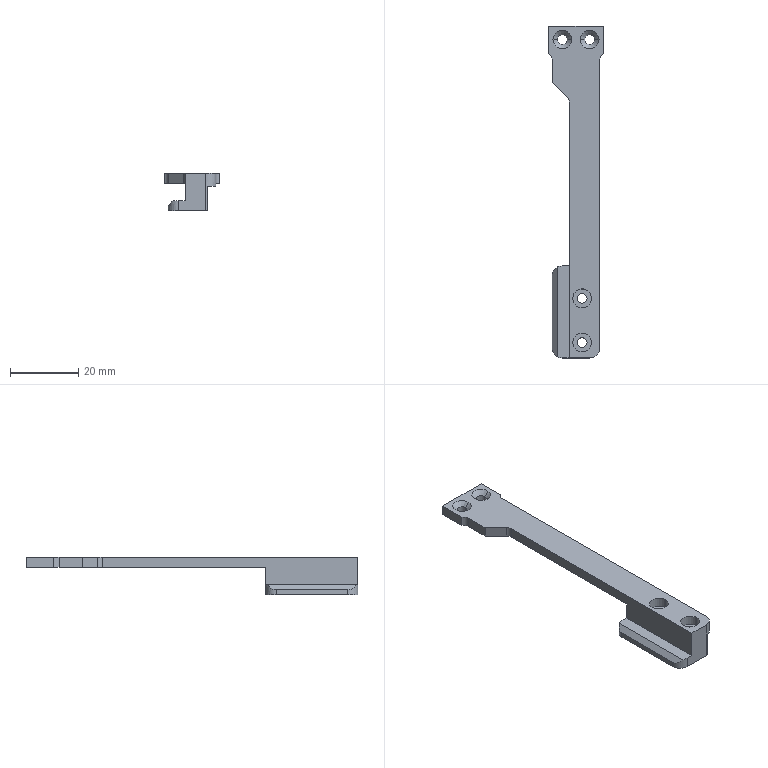NC program | NX | posted with a generic post | part box 16 x 97.4 x 11 mm
Whole program:
N10 G17 G21 G94 G90
(PLANAR_MILL , TOOL : D50面刀)
N12 T01 M6
N14 G53
N16 G17 G0 G90 X82.5 Y0. S4500 M3
N18 G43 Z20. H1
N20 Z2.
N22 G94 G1 Z0. F1000.
N24 X52.5
N26 X-52.5
N28 X-82.5
N30 Z2.
N32 G0 Z20.
N34 M5
(ADAPTIVE_MILLING , TOOL : D8-25-D8-60-3T-ROUGH)
N36 T02 M6
N38 G53
N40 G17 G0 G90 X-46.402 Y19.028 S6500 M3
N42 G43 Z20. H2
N44 Z-9.
N46 G94 G1 X-46.392 Y18.879 Z-9.937 F3000.
N48 X-46.383 Y18.729 Z-10.308
N50 X-46.373 Y18.579 Z-10.58
N52 X-46.364 Y18.429 Z-10.8
N54 X-46.354 Y18.28 Z-10.984
N56 X-46.345 Y18.13 Z-11.142
N58 X-46.335 Y17.98 Z-11.28
N60 X-46.326 Y17.831 Z-11.4
N62 X-46.316 Y17.681 Z-11.505
N64 X-46.306 Y17.531 Z-11.598
N66 X-46.297 Y17.382 Z-11.679
N68 X-46.287 Y17.232 Z-11.75
N70 X-46.278 Y17.082 Z-11.81
N72 X-46.268 Y16.932 Z-11.862
N74 X-46.259 Y16.783 Z-11.905
N76 X-46.249 Y16.633 Z-11.939
N78 X-46.24 Y16.483 Z-11.966
N80 X-46.23 Y16.334 Z-11.985
N82 X-46.221 Y16.184 Z-11.996
N84 X-46.211 Y16.034 Z-12.
N86 X-46.127 Y14.717
N88 G3 X-45.678 Y14.044 R0.808
N90 X-44.706 Y13.718 R3.559
N92 X-42.222 Y13.429 R17.156
N94 X-37.674 Y13.316 R97.009
N96 X-30.871 Y13.3 R763.382
N98 G1 X50.416 Y13.298
N100 G2 X52.463 Y12.608 R3.969
N102 X54.236 Y10.667 R5.764
N104 X55.257 Y7.88 R9.538
N106 X55.661 Y4.583 R22.23
N108 X55.783 Y0.035 R94.426
N110 X55.794 Y-8.015 R791.493
N112 X54.909 Y-10.261 R4.102
N114 X52.73 Y-11.98 R6.13
N116 X49.897 Y-12.857 R10.685
N118 X46.416 Y-13.198 R27.086
N120 X40.642 Y-13.292 R152.341
N122 G1 X34.517 Y-13.299
N124 X-50.405 Y-13.298
N126 G2 X-52.672 Y-12.474 R4.03
N128 X-54.396 Y-10.394 R5.971
N130 X-55.306 Y-7.66 R10.142
N132 X-55.685 Y-4.184 R24.685
N134 X-55.79 Y0.89 R120.171
N136 X-55.795 Y7.977 R799.405
N138 X-54.931 Y10.231 R4.082
N140 X-52.83 Y11.929 R6.022
N142 X-50.008 Y12.837 R10.358
N144 X-46.612 Y13.046 R12.952
N146 X-43.267 Y12.812 R655.851
N148 G3 X-36.446 Y12.619 R126.041
N150 X-28.071 Y12.6 R886.745
N152 G1 X48.054
N154 G2 X52.13 Y10.86 R5.749
N156 X53.837 Y8.22 R8.021
N158 X54.677 Y5.011 R13.845
N160 X55.015 Y0.827 R36.965
N162 X55.092 Y-5.734 R199.467
N164 X53.412 Y-9.583 R5.707
N166 X51.744 Y-10.847 R7.544
N168 G1 X51.634 Y-10.935
N170 X51.226 Y-11.293
N172 X50.775 Y-11.594
N174 X50.288 Y-11.834
N176 X49.774 Y-12.009
N178 G2 X47.766 Y-12.299 R17.026
N180 X42.698 Y-12.552 R62.148
N182 X32.198 Y-12.599 R684.903
N184 G1 X-48.088
N186 G2 X-52.094 Y-10.904 R5.706
N188 X-53.851 Y-8.193 R7.99
N190 X-54.696 Y-4.892 R14.186
N192 X-55.025 Y-0.531 R39.592
N194 X-55.091 Y5.768 R209.536
N196 X-53.4 Y9.598 R5.703
N198 X-50.192 Y11.518 R7.881
N200 X-47.097 Y12.055 R12.577
N202 X-43.423 Y12.069 R43.051
N204 G3 X-30.768 Y11.912 R366.289
N206 G1 X-24.818 Y11.911
N208 X-19.146 Y11.901
N210 X39.216 Y11.904
N212 X39.313 Y11.91
N214 X39.405 Y11.943
N216 G2 X40.7 Y12.15 R4.458
N218 G1 X48.7
N220 X49.242 Y12.114
N222 X49.774 Y12.008
N224 X50.288 Y11.834
N226 X50.775 Y11.594
N228 X51.227 Y11.292
N230 X51.635 Y10.934
N232 X51.993 Y10.526
N234 X52.294 Y10.075
N236 G2 X52.786 Y8.932 R7.946
N238 X54.029 Y3.576 R22.29
N240 X54.33 Y-1.313 R54.903
N242 X54.36 Y-4.113 R55.856
N244 X53.079 Y-7.871 R6.816
N246 G3 X52.823 Y-8.409 R1.194
N248 G1 X52.814 Y-8.542
N250 X52.708 Y-9.074
N252 X52.534 Y-9.588
N254 X52.294 Y-10.075
N256 X51.992 Y-10.527
N258 X51.634 Y-10.935
N260 X51.226 Y-11.293
N262 X50.775 Y-11.594
N264 X50.288 Y-11.834
N266 X49.774 Y-12.009
N268 X49.241 Y-12.115
N270 X48.7 Y-12.15
N272 X40.7
N274 G2 X39.504 Y-12.058 R26.192
N276 G3 X34.834 Y-11.917 R75.914
N278 X27.755 Y-11.912 R915.533
N280 G1 X21.195 Y-11.91
N282 X14.543 Y-11.911
N284 X8.855 Y-11.912
N286 X2.295 Y-11.91
N288 X-4.357 Y-11.911
N290 X-10.045 Y-11.912
N292 X-16.605 Y-11.91
N294 X-23.257 Y-11.911
N296 X-28.945 Y-11.912
N298 X-35.505 Y-11.91
N300 X-42.157 Y-11.911
N302 G2 X-46.445 Y-11.902 R363.082
N304 X-50.076 Y-10.787 R6.809
N306 X-52.479 Y-8.132 R7.677
N308 X-53.689 Y-4.851 R12.044
N310 X-54.21 Y-0.952 R26.009
N312 X-54.362 Y3.945 R78.972
N314 X-53.167 Y7.724 R6.66
N316 X-50.369 Y10.046 R7.311
N318 X-47.109 Y11.013 R11.338
N320 X-44.615 Y11.244 R19.109
N322 X-40.24 Y11.268 R90.415
N324 G3 X-26.496 Y11.211 R972.598
N326 G1 X-20.369 Y11.202
N328 X36.591 Y11.201
N330 G3 X37.866 Y11.22 R30.407
N332 X38.31 Y11.393 R0.897
N334 G2 X39.403 Y11.942 R4.489
N336 G3 X39.881 Y12.46 R0.8
N338 G1 X39.92 Y12.593
N340 X40.368 Y14.103 Z-11.9
N342 X40.428 Y14.308 F15000.
N344 X40.493 Y14.512
N346 G2 X41.176 Y15.012 R0.8
N348 G1 X42.32 Y15.099
N350 X43.465 Y15.18
N352 G2 X47.041 Y14.962 R15.611
N354 G1 X49.465 Y14.531
N356 G2 X52.242 Y13.617 R10.349
N358 X54.18 Y11.619 R4.161
N360 X54.698 Y10.453 R30.613
N362 X55.672 Y7.475 R20.843
N364 X56.453 Y3.624 R48.181
N366 G1 X56.843 Y1.191
N368 G2 X56.894 Y-3.677 R16.419
N370 X55.7 Y-8.423 R22.696
N372 G1 X55.145 Y-9.922
N374 G2 X53.588 Y-12.351 R6.749
N376 G1 X53.345 Y-12.594
N378 X53.1 Y-12.835
N380 G2 X51.435 Y-13.927 R5.954
N382 X49.324 Y-14.539 R8.216
N384 X47.858 Y-14.649 R9.488
N386 G1 X42.768 Y-14.633
N388 G2 X42.121 Y-14.301 R0.8
N390 G1 X41.995 Y-14.126
N392 X41.072 Y-12.849 Z-12. F3000.
N394 X40.783 Y-12.448
N396 G3 X40.261 Y-12.127 R0.8
N398 G2 X39.16 Y-11.847 R4.176
N400 G3 X37.181 Y-11.461 R10.069
N402 X33.309 Y-11.254 R43.648
N404 X24.798 Y-11.211 R537.488
N406 G1 X-43.627
N408 G2 X-45.64 Y-11.15 R20.214
N410 X-46.829 Y-11.06 R7.518
N412 G1 X-47.597 Y-10.894
N414 X-48.277 Y-10.669
N416 X-48.931 Y-10.378
N418 X-49.553 Y-10.023
N420 X-50.136 Y-9.608
N422 X-50.674 Y-9.136
N424 X-51.163 Y-8.613
N426 X-51.597 Y-8.043
N428 X-51.972 Y-7.433
N430 X-52.284 Y-6.789
N432 X-52.53 Y-6.116
N434 G2 X-53.436 Y-0.759 R28.799
N436 X-53.588 Y2.561 R37.75
N438 X-52.928 Y5.617 R7.487
N440 X-52.363 Y6.603 R7.056
N442 G3 X-52.232 Y6.908 R1.505
N444 G1 X-51.892 Y7.575
N446 X-51.484 Y8.203
N448 X-51.013 Y8.784
N450 X-50.484 Y9.314
N452 X-49.902 Y9.785
N454 X-49.275 Y10.192
N456 X-48.608 Y10.532
N458 X-47.909 Y10.8
N460 X-47.186 Y10.994
N462 X-46.668 Y11.076
N464 G3 X-46.418 Y12.573 R0.8
N466 X-46.768 Y12.669 Z-11.977 R0.911
N468 G1 X-47.968 Y12.821 Z-11.9
N470 X-49.193 Y12.976 F15000.
N472 G3 X-49.737 Y12.848 R0.801
N474 G1 X-51.376 Y11.756
N476 G3 X-52.999 Y10.279 R7.361
N478 X-53.965 Y8.863 R9.48
N480 G1 X-54.923 Y7.143
N482 G3 X-55.799 Y4.695 R7.904
N484 X-55.906 Y3.397 R7.242
N486 G1 X-55.895 Y1.82
N488 X-55.88 Y0.244
N490 X-55.858 Y-0.925
N492 X-55.826 Y-2.093
N494 X-55.776 Y-3.651
N496 G3 X-55.61 Y-4.113 R0.801
N498 G1 X-54.727 Y-5.259
N500 X-54.131 Y-6.031 Z-11.962 F3000.
N502 G3 X-53.628 Y-6.332 Z-12. R0.801
N504 X-52.707 Y-5.423 R0.8
N506 G1 X-52.814 Y-4.715
N508 X-52.85 Y-4.
N510 Y4.
N512 X-52.811 Y4.748
N514 X-52.694 Y5.487
N516 X-52.5 Y6.21
N518 X-52.232 Y6.908
N520 X-51.892 Y7.575
N522 X-51.484 Y8.203
N524 X-51.013 Y8.784
N526 X-50.484 Y9.314
N528 X-49.902 Y9.785
N530 X-49.275 Y10.192
N532 X-48.608 Y10.532
N534 X-47.909 Y10.8
N536 X-47.186 Y10.994
N538 X-46.447 Y11.111
N540 X-45.7 Y11.15
N542 X-24.7
N544 X-23.947 Y11.11
N546 X-23.203 Y10.992
N548 G3 X-21.366 Y10.7 R10.842
N550 X-17.093 Y10.529 R58.413
N552 X-9.784 Y10.501 R702.079
N554 G1 X29.679
N556 G3 X30.058 Y10.594 R0.885
N558 G1 X30.545 Y10.834
N560 X31.059 Y11.009
N562 X31.592 Y11.114
N564 X32.133 Y11.15
N566 X37.708
N568 G3 X38.296 Y11.382 R0.885
N570 X37.751 Y12.956 R0.88
N572 G1 X32.182 Y12.93
N574 X30.607 Y12.923 Z-11.9
N576 X-21.903 Y12.68 F15000.
N578 X-22.377 Y12.679 Z-11.93 F3000.
N580 X-22.851 Y12.673 Z-11.96
N582 G3 X-23.415 Y12.43 Z-12. R0.88
N584 X-23.034 Y10.946 R0.88
N586 G1 X-22.475 Y10.795
N588 G3 X-21.284 Y10.376 R10.102
N590 X-18.624 Y9.989 R15.901
N592 X-13.776 Y9.825 R80.03
N594 X-7.159 Y9.802 R706.917
N596 G1 X27.657
N598 G3 X28.961 Y9.88 R8.911
N600 X29.317 Y10.038 R1.004
N602 G1 X29.607 Y10.293
N604 X30.044 Y10.584
N606 G3 X30.324 Y11.743 R0.88
N608 X29.555 Y12.196 Z-11.941 R0.88
N610 G1 X28.915 Z-11.9
N612 X-20.696 Y12.186 F15000.
N614 X-21.054 Y12.187 Z-11.923 F3000.
N616 X-21.412 Y12.184 Z-11.945
N618 G3 X-22.122 Y11.764 Z-12. R0.88
N620 X-21.773 Y10.523 R0.88
N622 X-20.751 Y10.019 R15.197
N624 X-18.845 Y9.527 R9.403
N626 X-15.327 Y9.215 R31.139
N628 X-8.639 Y9.107 R177.423
N630 G1 X-4.796 Y9.102
N632 X26.157 Y9.103
N634 G3 X27.842 Y9.182 R15.371
N636 X28.525 Y9.335 R2.58
N638 X28.732 Y9.468 R1.803
N640 G2 X29.33 Y10.05 R9.159
N642 G3 X29.518 Y11.141 R0.88
N644 X28.754 Y11.592 Z-11.941 R0.88
N646 G1 X28.109 Y11.594 Z-11.9
N648 X-19.968 Y11.792 F15000.
N650 X-20.616 Y11.795 Z-11.941 F3000.
N652 G3 X-21.383 Y11.353 Z-12. R0.88
N654 X-21.102 Y10.179 R0.88
N656 X-20.29 Y9.659 R17.383
N658 X-18.517 Y9.038 R6.961
N660 X-15.312 Y8.609 R21.922
N662 X-10.183 Y8.432 R89.515
N664 X-2.521 Y8.402 R733.617
N666 G1 X24.673 Y8.403
N668 G3 X26.915 Y8.495 R22.789
N670 X27.862 Y8.686 R4.037
N672 X28.088 Y8.823 R1.617
N674 G1 X28.768 Y9.504
N676 G3 X28.909 Y10.565 R0.88
N678 X28.152 Y11.006 Z-11.942 R0.883
N680 G1 X27.493 Y11.011 Z-11.9
N682 X-19.264 Y11.323 F15000.
N684 X-19.909 Y11.327 Z-11.941 F3000.
N686 G3 X-20.679 Y10.884 Z-12. R0.88
N688 X-20.472 Y9.766 R0.88
N690 G1 X-19.93 Y9.323
N692 G3 X-18.391 Y8.609 R5.466
N694 X-15.594 Y8.062 R15.768
N696 X-11.092 Y7.781 R52.593
N698 X-2.78 Y7.704 R329.295
N700 G1 X1.417 Y7.702
N702 X22.762 Y7.703
N704 G3 X25.767 Y7.78 R40.305
N706 X27.147 Y8.005 R6.74
N708 X27.436 Y8.171 R1.061
N710 G1 X28.116 Y8.852
N712 G3 X28.258 Y9.91 R0.88
N714 X27.504 Y10.354 Z-11.942 R0.883
N716 G1 X26.845 Y10.362 Z-11.9
N718 X-18.716 Y10.877 F15000.
N720 X-19.363 Y10.884 Z-11.941 F3000.
N722 G3 X-20.133 Y10.447 Z-12. R0.88
N724 X-19.93 Y9.323 R0.88
N726 G1 X-19.581 Y8.978
N728 G3 X-18.305 Y8.222 R4.452
N730 X-15.83 Y7.558 R11.893
N732 X-11.884 Y7.164 R34.848
N734 X-5.389 Y7.019 R146.421
N736 X2.992 Y7.003 R929.816
N738 G1 X21.101
N740 G3 X24.752 Y7.075 R59.004
N742 X26.441 Y7.323 R8.305
N744 X26.76 Y7.495 R1.043
N746 G1 X27.44 Y8.176
N748 G3 X27.584 Y9.231 R0.88
N750 X26.833 Y9.678 Z-11.942 R0.883
N752 G1 X26.173 Y9.69 Z-11.9
N754 X-18.278 Y10.465 F15000.
N756 X-18.63 Y10.472 Z-11.922 F3000.
N758 X-18.981 Y10.475 Z-11.945
N760 G3 X-19.705 Y10.057 Z-12. R0.88
N762 X-19.581 Y8.978 R0.88
N764 G2 X-19.249 Y8.616 R2.829
N766 G3 X-18.208 Y7.854 R3.674
N768 X-16.049 Y7.098 R9.193
N770 X-12.557 Y6.588 R24.686
N772 X-6.846 Y6.349 R84.86
N774 X5.004 Y6.303 R901.745
N776 G1 X20.05
N778 G3 X23.888 Y6.378 R65.949
N780 X25.602 Y6.602 R10.161
N782 X26.082 Y6.817 R1.095
N784 G1 X26.762 Y7.498
N786 G3 X26.908 Y8.549 R0.88
N788 X26.161 Y9. Z-11.942 R0.883
N790 G1 X25.499 Y9.016 Z-11.9
N792 X-17.857 Y10.03 F15000.
N794 X-18.219 Y10.039 Z-11.923 F3000.
N796 X-18.582 Y10.045 Z-11.946
N798 G3 X-19.297 Y9.65 Z-12. R0.88
N800 X-19.249 Y8.616 R0.88
N802 X-18.765 Y8.025 R15.651
N804 X-17.547 Y7.184 R4.353
N806 X-15.14 Y6.39 R10.85
N808 X-13.824 Y6.15 R22.321
N810 G1 X24.851
N812 G3 X25.386 Y6.235 R2.074
N814 X25.661 Y6.397 R1.09
N816 G1 X26.094 Y6.83
N818 G3 X24.977 Y8.18 R0.88
N820 G1 X24.356 Y7.758
N822 G3 X24.851 Y6.15 R0.88
N824 X25.388 Y6.214 R1.326
N826 X25.644 Y6.382 R0.947
N828 X25.887 Y7.15 R0.8
N830 G1 X25.819 Y7.455
N832 X25.473 Y8.992 Z-11.9
N834 X25.443 Y9.124 F15000.
N836 X25.417 Y9.257
N838 G2 X25.644 Y9.926 R0.8
N840 G1 X27.387 Y11.669
N842 G2 X29.853 Y13.087 R5.458
N844 X32.738 Y13.66 R23.744
N846 G1 X34.093 Y13.843
N848 X35.45 Y14.022
N850 G2 X41.543 Y14.58 R89.585
N852 G1 X46.414 Y14.859
N854 G2 X49.514 Y14.541 R9.839
N856 X52.167 Y13.601 R15.696
N858 G1 X53.452 Y13.011
N860 G2 X53.759 Y11.805 R0.8
N862 G1 X53.63 Y11.633
N864 X52.686 Y10.371 Z-12. F3000.
N866 G3 X52.493 Y9.893 R0.845
N868 X52.534 Y9.588 R0.808
N870 G1 X52.709 Y9.074
N872 X52.815 Y8.541
N874 G3 X53.114 Y5.362 R42.02
N876 G2 X53.615 Y-2.142 R71.446
N878 G1 Y-4.755
N880 G2 X53.484 Y-5.17 R1.258
N882 G1 X52.899 Y-6.492
N884 G3 X52.85 Y-6.717 R2.433
N886 G1 Y-8.
N888 X52.821 Y-8.437
N890 G3 X53.767 Y-9.275 R0.8
N892 X54.282 Y-8.938 Z-11.96 R0.806
N894 G1 X54.811 Y-8.157 Z-11.9
N896 X55.369 Y-7.333 F15000.
N898 G3 X55.507 Y-6.886 R0.801
N900 G1 X55.536 Y6.449
N902 G3 X55.391 Y6.91 R0.801
N904 G1 X54.822 Y7.721
N906 X54.305 Y8.459 Z-11.957 F3000.
N908 G3 X53.743 Y8.794 Z-12. R0.8
N910 X52.85 Y8. R0.8
N912 G1 Y0.737
N914 G2 X52.887 Y-2.189 R70.707
N916 G1 X52.85 Y-2.72
N918 Y-6.745
N920 G3 X54.213 Y-7.313 R0.8
N922 X54.402 Y-7.017 Z-11.978 R0.805
N924 G1 X54.818 Y-5.868 Z-11.9
N926 X55.309 Y-4.51 F15000.
N928 G3 X55.356 Y-4.238 R0.812
N930 G1 Y-1.769
N932 G3 X55.309 Y-1.497 R0.812
N934 G1 X54.821 Y-0.148
N936 X54.402 Y1.009 Z-11.978 F3000.
N938 G3 X54.22 Y1.299 Z-12. R0.806
N940 X52.85 Y0.737 R0.8
N942 G1 Y-2.763
N944 G3 X53.212 Y-3.432 R0.8
N946 G1 X53.5 Y-3.621
N948 X54.818 Y-4.484 Z-11.9
N950 X54.94 Y-4.563 F15000.
N952 X55.059 Y-4.646
N954 G2 X55.356 Y-5.269 R0.8
N956 G1 Y-8.222
N958 G2 X54.893 Y-10.316 R5.041
N960 X53.998 Y-11.803 R7.279
N962 G1 X53.642 Y-12.261
N964 X53.282 Y-12.716
N966 G2 X51.56 Y-13.972 R4.554
N968 X50.057 Y-14.348 R5.057
N970 X46.725 Y-14.622 R120.723
N972 G1 X45.94 Y-14.67
N974 X45.154 Y-14.712
N976 X40.932 Y-14.917
N978 G2 X40.116 Y-14.309 R0.8
N980 G1 X40.063 Y-14.092
N982 X39.686 Y-12.562 Z-12. F3000.
N984 X39.657 Y-12.445
N986 X39.625 Y-12.328
N988 G3 X39.16 Y-11.847 R0.8
N990 G2 X38.568 Y-11.559 R3.884
N992 G3 X37.454 Y-11.152 R4.266
N994 G1 X-45.691 Y-11.15
N996 G3 X-46.571 Y-12.03 R0.88
N998 X-45.695 Y-12.91 R0.88
N1000 G1 X8.024 Y-13.113
N1002 X9.599 Y-13.119 Z-11.9
N1004 X37.516 Y-13.225 F15000.
N1006 X38.168 Y-13.227 Z-11.941 F3000.
N1008 G3 X38.933 Y-12.788 Z-12. R0.88
N1010 X38.643 Y-11.604 R0.88
N1012 G2 X38.134 Y-11.265 R8.397
N1014 G3 X37.708 Y-11.15 R0.868
N1016 G1 X37.358
N1018 G3 X36.608 Y-11.657 R0.808
N1020 G1 X36.226 Y-12.612
N1022 G2 X35.476 Y-13.119 R0.808
N1024 G1 X35.326 Z-11.996
N1026 X35.176 Z-11.985
N1028 X35.026 Z-11.966
N1030 X34.876 Z-11.939
N1032 X34.726 Z-11.905
N1034 X34.576 Z-11.862
N1036 X34.426 Z-11.81
N1038 X34.276 Z-11.75
N1040 X34.126 Z-11.679
N1042 X33.976 Z-11.598
N1044 X33.826 Z-11.505
N1046 X33.676 Z-11.4
N1048 X33.526 Z-11.28
N1050 X33.376 Z-11.142
N1052 X33.226 Z-10.984
N1054 X33.076 Z-10.8
N1056 X32.926 Z-10.58
N1058 X32.776 Z-10.308
N1060 X32.626 Z-9.937
N1062 X32.476 Z-9.
N1064 G0 Z20.
N1066 X-15.046 Y10.372
N1068 Z-9.
N1070 G1 X-15.196 Y10.364 Z-9.937
N1072 X-15.346 Y10.357 Z-10.308
N1074 X-15.496 Y10.349 Z-10.58
N1076 X-15.646 Y10.342 Z-10.8
N1078 X-15.796 Y10.334 Z-10.984
N1080 X-15.945 Y10.327 Z-11.142
N1082 X-16.095 Y10.319 Z-11.28
N1084 X-16.245 Y10.312 Z-11.4
N1086 X-16.395 Y10.305 Z-11.505
N1088 X-16.545 Y10.297 Z-11.598
N1090 X-16.694 Y10.29 Z-11.679
N1092 X-16.844 Y10.282 Z-11.75
N1094 X-16.994 Y10.275 Z-11.81
N1096 X-17.144 Y10.267 Z-11.862
N1098 X-17.294 Y10.26 Z-11.905
N1100 X-17.444 Y10.253 Z-11.939
N1102 X-17.593 Y10.245 Z-11.966
N1104 X-17.743 Y10.238 Z-11.985
N1106 X-17.893 Y10.23 Z-11.996
N1108 X-18.043 Y10.223 Z-12.
N1110 G3 X-18.787 Y9.612 R0.808
N1112 G1 X-18.991 Y8.796
N1114 G3 X-18.888 Y8.164 R0.808
N1116 X-18.419 Y7.511 R4.079
N1118 X-17.057 Y6.569 R4.771
N1120 X-16.125 Y6.183 R9.402
N1122 G1 X-15.952 Y6.15
N1124 X-13.764
N1126 G3 X-12.976 Y7.421 R0.88
N1128 X-13.512 Y7.873 Z-11.954 R0.885
N1130 G1 X-14.33 Y8.118 Z-11.9
N1132 X-17.035 Y8.927 F15000.
N1134 X-17.659 Y9.113 Z-11.941 F3000.
N1136 G3 X-18.517 Y8.908 Z-12. R0.88
N1138 X-18.652 Y7.796 R0.88
N1140 G2 X-18.404 Y7.373 R2.829
N1142 G3 X-17.494 Y6.466 R3.324
N1144 X-16.956 Y6.175 R1.735
N1146 G1 X-16.806 Y6.15
N1148 X-15.931
N1150 G3 X-15.064 Y7.175 R0.88
N1152 X-15.579 Y7.836 Z-11.945 R0.883
N1154 G1 X-16.222 Y8.117 Z-11.9
N1156 X-16.669 Y8.313 F15000.
N1158 X-17.264 Y8.573 Z-11.941 F3000.
N1160 G3 X-18.142 Y8.473 Z-12. R0.88
N1162 X-18.404 Y7.373 R0.88
N1164 G1 X-18.169 Y6.903
N1166 G3 X-17.593 Y6.274 R2.
N1168 X-17.204 Y6.15 R0.98
N1170 G1 X-16.766
N1172 G3 X-16.416 Y7.837 R0.88
N1174 G1 X-17.032 Y8.104
N1176 G3 X-18.169 Y6.903 R0.88
N1178 G1 X-18.039 Y6.595
N1180 G3 X-17.296 Y6.15 R0.845
N1182 G1 X-17.121
N1184 G3 X-16.321 Y7.071 R0.808
N1186 G1 X-16.469 Y8.119
N1188 X-16.49 Y8.268 Z-11.996
N1190 X-16.511 Y8.416 Z-11.985
N1192 X-16.532 Y8.565 Z-11.966
N1194 X-16.554 Y8.713 Z-11.939
N1196 X-16.575 Y8.862 Z-11.905
N1198 X-16.596 Y9.01 Z-11.862
N1200 X-16.617 Y9.159 Z-11.81
N1202 X-16.638 Y9.307 Z-11.75
N1204 X-16.659 Y9.456 Z-11.679
N1206 X-16.68 Y9.604 Z-11.598
N1208 X-16.701 Y9.753 Z-11.505
N1210 X-16.722 Y9.901 Z-11.4
N1212 X-16.743 Y10.05 Z-11.28
N1214 X-16.764 Y10.198 Z-11.142
N1216 X-16.785 Y10.347 Z-10.984
N1218 X-16.806 Y10.495 Z-10.8
N1220 X-16.827 Y10.644 Z-10.58
N1222 X-16.848 Y10.792 Z-10.308
N1224 X-16.869 Y10.941 Z-9.937
N1226 X-16.89 Y11.089 Z-9.
N1228 G0 Z20.
(ADAPTIVE_MILLING_COPY , TOOL : D8-25-D8-60-3T-ROUGH)
N1230 X-57.78 Y0.242
N1232 Z-4.85
N1234 G1 X-57.632 Y0.266 Z-5.787
N1236 X-57.484 Y0.29 Z-6.158
N1238 X-57.335 Y0.314 Z-6.43
N1240 X-57.187 Y0.338 Z-6.65
N1242 X-57.039 Y0.362 Z-6.834
N1244 X-56.891 Y0.386 Z-6.992
N1246 X-56.743 Y0.411 Z-7.13
N1248 X-56.595 Y0.435 Z-7.25
N1250 X-56.447 Y0.459 Z-7.355
N1252 X-56.299 Y0.483 Z-7.448
N1254 X-56.151 Y0.507 Z-7.529
N1256 X-56.003 Y0.531 Z-7.6
N1258 X-55.855 Y0.555 Z-7.66
N1260 X-55.707 Y0.579 Z-7.712
N1262 X-55.559 Y0.603 Z-7.755
N1264 X-55.411 Y0.627 Z-7.789
N1266 X-55.263 Y0.651 Z-7.816
N1268 X-55.115 Y0.675 Z-7.835
N1270 X-54.967 Y0.7 Z-7.846
N1272 X-54.819 Y0.724 Z-7.85
N1274 X-53.528 Y0.934
N1276 G3 X-52.849 Y1.731 R0.808
N1278 G2 X-52.619 Y3.365 R4.604
N1280 X-51.945 Y5.342 R19.07
N1282 X-49.932 Y8.166 R7.591
N1284 X-47.33 Y9.587 R7.546
N1286 X-44.245 Y10.199 R14.819
N1288 X-40.051 Y10.412 R50.021
N1290 X-31.652 Y10.45 R543.432
N1292 X-26.196 Y10.44 R435.149
N1294 X-23.362 Y9.952 R9.242
N1296 X-20.651 Y8.229 R7.471
N1298 X-19.443 Y7.016 R224.252
N1300 G3 X-18.439 Y6.235 R5.055
N1302 X-18.122 Y6.15 R1.075
N1304 G1 X-17.247
N1306 G3 X-16.475 Y6.738 R0.8
N1308 X-16.598 Y7.418 Z-7.805 R0.805
N1310 G1 X-17.101 Y8.116 Z-7.75
N1312 X-18.081 Y9.476 F15000.
N1314 X-18.121 Y9.526
N1316 X-18.164 Y9.574
N1318 X-18.395 Y9.806
N1320 X-18.63 Y10.035
N1322 G3 X-19.278 Y10.53 R4.311
N1324 G1 X-20.008 Y10.986
N1326 X-20.742 Y11.437
N1328 G3 X-22.76 Y12.314 R9.095
N1330 X-24.201 Y12.584 R7.625
N1332 G1 X-25.344 Y12.684
N1334 X-26.487 Y12.774
N1336 G3 X-29.105 Y12.907 R71.653
N1338 G1 X-35.996 Y13.131
N1340 G3 X-43.828 Y12.688 R44.113
N1342 G1 X-44.624 Y12.572
N1344 X-45.42 Y12.451
N1346 G3 X-50.148 Y10.963 R17.847
N1348 G1 X-50.588 Y10.754
N1350 X-51.026 Y10.541
N1352 G3 X-53.482 Y8.122 R5.861
N1354 G1 X-54.391 Y6.434
N1356 G3 X-54.48 Y5.95 R0.801
N1358 G1 X-54.289 Y4.498
N1360 X-54.162 Y3.539 Z-7.811 F3000.
N1362 G3 X-53.872 Y3.021 Z-7.85 R0.8
N1364 X-52.619 Y3.365 R0.8
N1366 G2 X-52.219 Y4.2 R5.047
N1368 X-50.736 Y6.094 R19.531
N1370 X-47.039 Y8.53 R9.468
N1372 X-43.47 Y9.372 R16.153
N1374 X-39.195 Y9.676 R43.365
N1376 X-31.67 Y9.748 R275.178
N1378 X-27.558 Y9.735 R190.549
N1380 X-24.879 Y9.358 R10.668
N1382 X-22.274 Y8.113 R9.666
N1384 X-20.406 Y6.785 R61.295
N1386 G3 X-19.494 Y6.221 R7.669
N1388 X-19.215 Y6.15 R1.307
N1390 G1 X-18.078
N1392 G3 X-17.315 Y6.708 R0.8
N1394 X-17.405 Y7.383 Z-7.805 R0.8
N1396 G1 X-17.877 Y8.116 Z-7.75
N1398 X-18.612 Y9.261 F15000.
N1400 G3 X-18.995 Y9.574 R0.801
N1402 G1 X-22.659 Y11.001
N1404 G3 X-26.442 Y11.957 R15.788
N1406 X-30.356 Y12.359 R92.331
N1408 X-34.284 Y12.399 R27.92
N1410 G1 X-41.655 Y11.956
N1412 G3 X-46.928 Y11.091 R26.082
N1414 X-50.857 Y9.324 R14.319
N1416 G1 X-52.831 Y8.05
N1418 G3 X-53.196 Y7.415 R0.8
N1420 G1 X-53.258 Y6.078
N1422 X-53.299 Y5.208 Z-7.805 F3000.
N1424 G3 X-53.037 Y4.578 Z-7.85 R0.8
N1426 X-51.913 Y4.626 R0.8
N1428 G2 X-51.154 Y5.347 R4.836
N1430 X-48.936 Y6.706 R36.392
N1432 X-44.164 Y8.378 R16.329
N1434 X-39.647 Y8.891 R33.34
N1436 X-33.262 Y9.038 R132.904
N1438 X-28.887 Y9.033 R185.583
N1440 X-25.944 Y8.646 R12.409
N1442 X-22.888 Y7.359 R13.485
N1444 G3 X-21.105 Y6.354 R103.956
N1446 X-20.601 Y6.156 R1.661
N1448 X-19.154 Y6.15 R44.718
N1450 X-18.355 Y7.003 R0.8
N1452 X-18.678 Y7.593 Z-7.806 R0.8
N1454 G1 X-19.387 Y8.117 Z-7.75
N1456 X-20.742 Y9.118 F15000.
N1458 G3 X-20.926 Y9.219 R0.85
N1460 G1 X-23.669 Y10.295
N1462 G3 X-27.837 Y11.364 R17.649
N1464 X-31.362 Y11.55 R22.075
N1466 G1 X-38.585 Y11.352
N1468 G3 X-43.791 Y10.863 R39.475
N1470 G1 X-44.339 Y10.775
N1472 X-44.886 Y10.683
N1474 G3 X-48.086 Y9.749 R16.188
N1476 G1 X-49.794 Y9.053
N1478 G3 X-50.118 Y8.811 R0.803
N1480 G1 X-51.04 Y7.655
N1482 X-51.68 Y6.851 Z-7.815 F3000.
N1484 G3 X-51.854 Y6.343 Z-7.85 R0.801
N1486 X-50.712 Y5.63 R0.8
N1488 G2 X-49.654 Y6.039 R4.744
N1490 G3 X-47.425 Y6.732 R58.634
N1492 G2 X-40.827 Y8.031 R30.548
N1494 X-34.972 Y8.305 R79.506
N1496 X-29.985 Y8.323 R135.921
N1498 X-24.303 Y7.054 R14.468
N1500 G1 X-22.448 Y6.214
N1502 G3 X-22.186 Y6.15 R1.555
N1504 G1 X-20.524
N1506 G3 X-19.728 Y7.033 R0.8
N1508 X-20.064 Y7.605 Z-7.807 R0.8
N1510 G1 X-20.793 Y8.117 Z-7.75
N1512 X-21.61 Y8.691 F15000.
N1514 G3 X-22.074 Y8.836 R0.801
N1516 G1 X-48.188 Y8.704
N1518 G3 X-48.618 Y8.576 R0.802
N1520 G1 X-49.385 Y8.081
N1522 X-50.323 Y7.476 Z-7.821 F3000.
N1524 G3 X-50.619 Y7.133 Z-7.85 R0.802
N1526 X-49.739 Y6.018 R0.8
N1528 G2 X-48.612 Y6.15 R4.791
N1530 G3 X-46.585 Y6.418 R16.153
N1532 G2 X-42.268 Y7.117 R76.734
N1534 X-35.811 Y7.56 R67.754
N1536 X-30.999 Y7.604 R96.322
N1538 X-25.266 Y6.507 R17.413
N1540 G1 X-24.343 Y6.175
N1542 X-24.195 Y6.15
N1544 X-22.182
N1546 G3 X-21.387 Y7.034 R0.8
N1548 X-21.723 Y7.605 Z-7.807 R0.8
N1550 G1 X-22.454 Y8.117 Z-7.75
N1552 X-23.274 Y8.691 F15000.
N1554 G3 X-23.733 Y8.836 R0.801
N1556 G1 X-47.062
N1558 G3 X-47.521 Y8.691 R0.801
N1560 G1 X-48.333 Y8.122
N1562 X-49.071 Y7.605 Z-7.807 F3000.
N1564 G3 X-49.407 Y7.044 Z-7.85 R0.8
N1566 X-48.612 Y6.15 R0.8
N1568 X-45.641 Y6.156 R263.886
N1570 X-42.506 Y6.412 R64.3
N1572 G2 X-32.196 Y6.884 R99.248
N1574 X-27.009 Y6.173 R20.625
N1576 G1 X-26.874 Y6.15
N1578 X-24.162
N1580 G3 X-23.908 Y7.709 R0.8
N1582 G1 X-25.43 Y8.118 Z-7.75
N1584 X-26.169 Y8.316 F15000.
N1586 X-26.261 Y8.334
N1588 X-26.354 Y8.343
N1590 X-44.262 Y8.836
N1592 G3 X-44.747 Y8.688 R0.801
N1594 G1 X-45.543 Y8.122
N1596 X-46.276 Y7.602 Z-7.807 F3000.
N1598 G3 X-46.608 Y7.035 Z-7.85 R0.8
N1600 X-45.812 Y6.15 R0.8
N1602 G1 X-26.825
N1604 G3 X-26.025 Y6.845 R0.808
N1606 G1 X-25.846 Y8.119
N1608 X-25.825 Y8.268 Z-7.846
N1610 X-25.804 Y8.416 Z-7.835
N1612 X-25.783 Y8.565 Z-7.816
N1614 X-25.762 Y8.713 Z-7.789
N1616 X-25.741 Y8.862 Z-7.755
N1618 X-25.72 Y9.01 Z-7.712
N1620 X-25.699 Y9.159 Z-7.66
N1622 X-25.679 Y9.307 Z-7.6
N1624 X-25.658 Y9.456 Z-7.529
N1626 X-25.637 Y9.604 Z-7.448
N1628 X-25.616 Y9.753 Z-7.355
N1630 X-25.595 Y9.902 Z-7.25
N1632 X-25.574 Y10.05 Z-7.13
N1634 X-25.553 Y10.199 Z-6.992
N1636 X-25.532 Y10.347 Z-6.834
N1638 X-25.511 Y10.496 Z-6.65
N1640 X-25.491 Y10.644 Z-6.43
N1642 X-25.47 Y10.793 Z-6.158
N1644 X-25.449 Y10.941 Z-5.787
N1646 X-25.428 Y11.09 Z-4.85
N1648 G0 Z20.
N1650 M5
(DRILLING , TOOL : 倒角D6-90度)
N1652 T03 M6
N1654 G53
N1656 G17 G0 G90 X-44.2 Y-1.799 S2500 M3
N1658 G43 Z20. H3
N1660 G94 G81 G99 Z-2.85 F200. R3.
N1662 X-31.2
N1664 G80
N1666 G0 X-31.2 Y-1.799 Z20.
(DRILLING_COPY , TOOL : 倒角D6-90度)
N1668 X44.7 Y-4.
N1670 G81 Z-2.75 F200. R3.
N1672 Y4.
N1674 G80
N1676 G0 X44.7 Y4. Z20.
(PLANAR_MILL_4 , TOOL : 倒角D6-90度)
N1678 X-52.798 Y8. S3000
N1680 Z-8.5
N1682 G1 Z-10.5 F600.
N1684 X-48.298
N1686 X-22.102
N1688 X-17.602
N1690 Z-8.5
N1692 G0 Z20.
(PLANAR_MILL_3_COPY_1 , TOOL : 倒角D6-90度)
N1694 X42.613 Y-11.992 S3500
N1696 Z0.5
N1698 G1 Z-1.5 F1000.
N1700 G41 X42.7 Y-11.5 D3
N1702 G3 X40.7 Y-9.5 R2.
N1704 G2 X39.401 Y-8.75 R1.5
N1706 G3 X38.968 Y-8.5 R0.5
N1708 G1 X-45.7
N1710 G2 X-50.2 Y-4. R4.5
N1712 G1 Y2.
N1714 G2 X-48.7 Y3.5 R1.5
N1716 G1 X26.305
N1718 G3 X26.658 Y3.646 R0.5
N1720 G1 X31.072 Y8.061
N1722 G2 X32.133 Y8.5 R1.5
N1724 G1 X38.968
N1726 G3 X39.401 Y8.75 R0.5
N1728 G2 X40.7 Y9.5 R1.5
N1730 G1 X48.7
N1732 G2 X50.2 Y8. R1.5
N1734 G1 Y-8.
N1736 G2 X48.7 Y-9.5 R1.5
N1738 G1 X40.7
N1740 G3 X38.7 Y-11.5 R2.
N1742 G40
N1744 G1 X38.787 Y-11.992
N1746 Z0.5
N1748 G0 Z20.
N1750 M5
(DRILLING_COPY_1 , TOOL : 钻头D2.9-39-67)
N1752 T04 M6
N1754 G53
N1756 G17 G0 G90 X-44.2 Y-1.799 S3000 M3
N1758 G43 Z20. H4
N1760 G94 G83 G99 Z-15. F200. Q2. R3.
N1762 X-31.2
N1764 G80
N1766 G0 X-31.2 Y-1.799 Z20.
(DRILLING_COPY_COPY , TOOL : 钻头D2.9-39-67)
N1768 X44.7 Y-4.
N1770 G81 Z-6. F200. R3.
N1772 Y4.
N1774 G80
N1776 G0 X44.7 Y4. Z20.
N1778 M5
(PLANAR_MILL_1 , TOOL : D3-9-D4-50-3T-ROUGH)
N1780 T05 M6
N1782 G53
N1784 G17 G0 G90 X-43.324 Y-0.96 S4500 M3
N1786 G43 Z20. H5
N1788 Z0.5
N1790 G94 G1 X-43.337 Y-0.936 Z0.499 F800.
N1792 X-43.931 Y-0.609 Z0.469
N1794 X-44.469 Z0.446
N1796 X-45.063 Y-0.936 Z0.416
N1798 X-45.39 Y-1.53 Z0.387
N1800 Y-2.068 Z0.363
N1802 X-45.063 Y-2.662 Z0.333
N1804 X-44.469 Y-2.989 Z0.304
N1806 X-43.931 Z0.28
N1808 X-43.337 Y-2.662 Z0.251
N1810 X-43.01 Y-2.068 Z0.221
N1812 Y-1.53 Z0.198
N1814 X-43.337 Y-0.936 Z0.168
N1816 X-43.931 Y-0.609 Z0.138
N1818 X-44.469 Z0.115
N1820 X-45.063 Y-0.936 Z0.085
N1822 X-45.39 Y-1.53 Z0.056
N1824 Y-2.068 Z0.032
N1826 X-45.063 Y-2.662 Z0.003
N1828 X-44.469 Y-2.989 Z-0.027
N1830 X-43.931 Z-0.05
N1832 X-43.337 Y-2.662 Z-0.08
N1834 X-43.01 Y-2.068 Z-0.11
N1836 Y-1.53 Z-0.133
N1838 X-43.337 Y-0.936 Z-0.163
N1840 X-43.931 Y-0.609 Z-0.192
N1842 X-44.469 Z-0.216
N1844 X-45.063 Y-0.936 Z-0.245
N1846 X-45.39 Y-1.53 Z-0.275
N1848 Y-2.068 Z-0.298
N1850 X-45.063 Y-2.662 Z-0.328
N1852 X-44.469 Y-2.989 Z-0.358
N1854 X-43.931 Z-0.381
N1856 X-43.337 Y-2.662 Z-0.411
N1858 X-43.01 Y-2.068 Z-0.44
N1860 Y-1.53 Z-0.464
N1862 X-43.337 Y-0.936 Z-0.493
N1864 X-43.931 Y-0.609 Z-0.523
N1866 X-44.469 Z-0.547
N1868 X-45.063 Y-0.936 Z-0.576
N1870 X-45.39 Y-1.53 Z-0.606
N1872 Y-2.068 Z-0.629
N1874 X-45.063 Y-2.662 Z-0.659
N1876 X-44.469 Y-2.989 Z-0.688
N1878 X-43.931 Z-0.712
N1880 X-43.337 Y-2.662 Z-0.741
N1882 X-43.01 Y-2.068 Z-0.771
N1884 Y-1.53 Z-0.795
N1886 X-43.337 Y-0.936 Z-0.824
N1888 X-43.931 Y-0.609 Z-0.854
N1890 X-44.469 Z-0.877
N1892 X-45.063 Y-0.936 Z-0.907
N1894 X-45.39 Y-1.53 Z-0.936
N1896 Y-2.068 Z-0.96
N1898 X-45.063 Y-2.662 Z-0.99
N1900 X-44.469 Y-2.989 Z-1.019
N1902 X-43.931 Z-1.043
N1904 X-43.337 Y-2.662 Z-1.072
N1906 X-43.01 Y-2.068 Z-1.102
N1908 Y-1.53 Z-1.125
N1910 X-43.337 Y-0.936 Z-1.155
N1912 X-43.931 Y-0.609 Z-1.185
N1914 X-44.469 Z-1.208
N1916 X-45.063 Y-0.936 Z-1.238
N1918 X-45.39 Y-1.53 Z-1.267
N1920 Y-2.068 Z-1.291
N1922 X-45.063 Y-2.662 Z-1.32
N1924 X-44.469 Y-2.989 Z-1.35
N1926 X-43.931 Z-1.373
N1928 X-43.337 Y-2.662 Z-1.403
N1930 X-43.01 Y-2.068 Z-1.433
N1932 Y-1.53 Z-1.456
N1934 X-43.337 Y-0.936 Z-1.486
N1936 X-43.931 Y-0.609 Z-1.515
N1938 X-44.469 Z-1.539
N1940 X-45.063 Y-0.936 Z-1.568
N1942 X-45.39 Y-1.53 Z-1.598
N1944 Y-2.068 Z-1.621
N1946 X-45.063 Y-2.662 Z-1.651
N1948 X-44.469 Y-2.989 Z-1.681
N1950 X-43.931 Z-1.704
N1952 X-43.337 Y-2.662 Z-1.734
N1954 X-43.01 Y-2.068 Z-1.763
N1956 Y-1.53 Z-1.787
N1958 X-43.337 Y-0.936 Z-1.816
N1960 X-43.931 Y-0.609 Z-1.846
N1962 X-44.469 Z-1.87
N1964 X-45.063 Y-0.936 Z-1.899
N1966 X-45.39 Y-1.53 Z-1.929
N1968 Y-2.068 Z-1.952
N1970 X-45.063 Y-2.662 Z-1.982
N1972 X-44.469 Y-2.989 Z-2.011
N1974 X-43.931 Z-2.035
N1976 X-43.337 Y-2.662 Z-2.064
N1978 X-43.01 Y-2.068 Z-2.094
N1980 Y-1.53 Z-2.118
N1982 X-43.337 Y-0.936 Z-2.147
N1984 X-43.931 Y-0.609 Z-2.177
N1986 X-44.469 Z-2.2
N1988 X-45.063 Y-0.936 Z-2.23
N1990 X-45.39 Y-1.53 Z-2.259
N1992 Y-2.068 Z-2.283
N1994 X-45.063 Y-2.662 Z-2.313
N1996 X-44.469 Y-2.989 Z-2.342
N1998 X-43.931 Z-2.366
N2000 X-43.337 Y-2.662 Z-2.395
N2002 X-43.01 Y-2.068 Z-2.425
N2004 Y-1.53 Z-2.448
N2006 X-43.337 Y-0.936 Z-2.478
N2008 X-43.931 Y-0.609 Z-2.508
N2010 X-44.469 Z-2.531
N2012 X-45.063 Y-0.936 Z-2.561
N2014 X-45.39 Y-1.53 Z-2.59
N2016 Y-2.068 Z-2.614
N2018 X-45.063 Y-2.662 Z-2.643
N2020 X-44.469 Y-2.989 Z-2.673
N2022 X-43.931 Z-2.696
N2024 X-43.337 Y-2.662 Z-2.726
N2026 X-43.01 Y-2.068 Z-2.756
N2028 Y-1.53 Z-2.779
N2030 X-43.337 Y-0.936 Z-2.809
N2032 X-43.931 Y-0.609 Z-2.838
N2034 X-44.2 Z-2.85
N2036 G3 X-45.39 Y-1.799 R1.19
N2038 X-44.2 Y-0.609 R-1.19
N2040 G1 Z-2.35
N2042 G0 Z20.
N2044 X-30.324 Y-0.96
N2046 Z0.5
N2048 G1 X-30.337 Y-0.936 Z0.499
N2050 X-30.931 Y-0.609 Z0.469
N2052 X-31.469 Z0.446
N2054 X-32.063 Y-0.936 Z0.416
N2056 X-32.39 Y-1.53 Z0.387
N2058 Y-2.068 Z0.363
N2060 X-32.063 Y-2.662 Z0.333
N2062 X-31.469 Y-2.989 Z0.304
N2064 X-30.931 Z0.28
N2066 X-30.337 Y-2.662 Z0.251
N2068 X-30.01 Y-2.068 Z0.221
N2070 Y-1.53 Z0.198
N2072 X-30.337 Y-0.936 Z0.168
N2074 X-30.931 Y-0.609 Z0.138
N2076 X-31.469 Z0.115
N2078 X-32.063 Y-0.936 Z0.085
N2080 X-32.39 Y-1.53 Z0.056
N2082 Y-2.068 Z0.032
N2084 X-32.063 Y-2.662 Z0.003
N2086 X-31.469 Y-2.989 Z-0.027
N2088 X-30.931 Z-0.05
N2090 X-30.337 Y-2.662 Z-0.08
N2092 X-30.01 Y-2.068 Z-0.11
N2094 Y-1.53 Z-0.133
N2096 X-30.337 Y-0.936 Z-0.163
N2098 X-30.931 Y-0.609 Z-0.192
N2100 X-31.469 Z-0.216
N2102 X-32.063 Y-0.936 Z-0.245
N2104 X-32.39 Y-1.53 Z-0.275
N2106 Y-2.068 Z-0.298
N2108 X-32.063 Y-2.662 Z-0.328
N2110 X-31.469 Y-2.989 Z-0.358
N2112 X-30.931 Z-0.381
N2114 X-30.337 Y-2.662 Z-0.411
N2116 X-30.01 Y-2.068 Z-0.44
N2118 Y-1.53 Z-0.464
N2120 X-30.337 Y-0.936 Z-0.493
N2122 X-30.931 Y-0.609 Z-0.523
N2124 X-31.469 Z-0.547
N2126 X-32.063 Y-0.936 Z-0.576
N2128 X-32.39 Y-1.53 Z-0.606
N2130 Y-2.068 Z-0.629
N2132 X-32.063 Y-2.662 Z-0.659
N2134 X-31.469 Y-2.989 Z-0.688
N2136 X-30.931 Z-0.712
N2138 X-30.337 Y-2.662 Z-0.741
N2140 X-30.01 Y-2.068 Z-0.771
N2142 Y-1.53 Z-0.795
N2144 X-30.337 Y-0.936 Z-0.824
N2146 X-30.931 Y-0.609 Z-0.854
N2148 X-31.469 Z-0.877
N2150 X-32.063 Y-0.936 Z-0.907
N2152 X-32.39 Y-1.53 Z-0.936
N2154 Y-2.068 Z-0.96
N2156 X-32.063 Y-2.662 Z-0.99
N2158 X-31.469 Y-2.989 Z-1.019
N2160 X-30.931 Z-1.043
N2162 X-30.337 Y-2.662 Z-1.072
N2164 X-30.01 Y-2.068 Z-1.102
N2166 Y-1.53 Z-1.125
N2168 X-30.337 Y-0.936 Z-1.155
N2170 X-30.931 Y-0.609 Z-1.185
N2172 X-31.469 Z-1.208
N2174 X-32.063 Y-0.936 Z-1.238
N2176 X-32.39 Y-1.53 Z-1.267
N2178 Y-2.068 Z-1.291
N2180 X-32.063 Y-2.662 Z-1.32
N2182 X-31.469 Y-2.989 Z-1.35
N2184 X-30.931 Z-1.373
N2186 X-30.337 Y-2.662 Z-1.403
N2188 X-30.01 Y-2.068 Z-1.433
N2190 Y-1.53 Z-1.456
N2192 X-30.337 Y-0.936 Z-1.486
N2194 X-30.931 Y-0.609 Z-1.515
N2196 X-31.469 Z-1.539
N2198 X-32.063 Y-0.936 Z-1.568
N2200 X-32.39 Y-1.53 Z-1.598
N2202 Y-2.068 Z-1.621
N2204 X-32.063 Y-2.662 Z-1.651
N2206 X-31.469 Y-2.989 Z-1.681
N2208 X-30.931 Z-1.704
N2210 X-30.337 Y-2.662 Z-1.734
N2212 X-30.01 Y-2.068 Z-1.763
N2214 Y-1.53 Z-1.787
N2216 X-30.337 Y-0.936 Z-1.816
N2218 X-30.931 Y-0.609 Z-1.846
N2220 X-31.469 Z-1.87
N2222 X-32.063 Y-0.936 Z-1.899
N2224 X-32.39 Y-1.53 Z-1.929
N2226 Y-2.068 Z-1.952
N2228 X-32.063 Y-2.662 Z-1.982
N2230 X-31.469 Y-2.989 Z-2.011
N2232 X-30.931 Z-2.035
N2234 X-30.337 Y-2.662 Z-2.064
N2236 X-30.01 Y-2.068 Z-2.094
N2238 Y-1.53 Z-2.118
N2240 X-30.337 Y-0.936 Z-2.147
N2242 X-30.931 Y-0.609 Z-2.177
N2244 X-31.469 Z-2.2
N2246 X-32.063 Y-0.936 Z-2.23
N2248 X-32.39 Y-1.53 Z-2.259
N2250 Y-2.068 Z-2.283
N2252 X-32.063 Y-2.662 Z-2.313
N2254 X-31.469 Y-2.989 Z-2.342
N2256 X-30.931 Z-2.366
N2258 X-30.337 Y-2.662 Z-2.395
N2260 X-30.01 Y-2.068 Z-2.425
N2262 Y-1.53 Z-2.448
N2264 X-30.337 Y-0.936 Z-2.478
N2266 X-30.931 Y-0.609 Z-2.508
N2268 X-31.469 Z-2.531
N2270 X-32.063 Y-0.936 Z-2.561
N2272 X-32.39 Y-1.53 Z-2.59
N2274 Y-2.068 Z-2.614
N2276 X-32.063 Y-2.662 Z-2.643
N2278 X-31.469 Y-2.989 Z-2.673
N2280 X-30.931 Z-2.696
N2282 X-30.337 Y-2.662 Z-2.726
N2284 X-30.01 Y-2.068 Z-2.756
N2286 Y-1.53 Z-2.779
N2288 X-30.337 Y-0.936 Z-2.809
N2290 X-30.931 Y-0.609 Z-2.838
N2292 X-31.2 Z-2.85
N2294 G3 X-32.39 Y-1.799 R1.19
N2296 X-31.2 Y-0.609 R-1.19
N2298 G1 Z-2.35
N2300 G0 Z20.
(PLANAR_MILL_1_COPY , TOOL : D3-9-D4-50-3T-ROUGH)
N2302 X-44.2 Y-1.549
N2304 Z-0.9
N2306 G1 Z-2.9 F600.
N2308 G41 X-43.2 D5
N2310 G3 X-44.2 Y-0.549 R1.
N2312 X-45.45 Y-1.799 R1.25
N2314 X-44.2 Y-0.549 R-1.25
N2316 X-45.2 Y-1.549 R1.
N2318 G40
N2320 G1 X-44.2
N2322 Z-0.9
N2324 G0 Z20.
N2326 X-31.2
N2328 Z-0.9
N2330 G1 Z-2.9
N2332 G41 X-30.2
N2334 G3 X-31.2 Y-0.549 R1.
N2336 X-32.45 Y-1.799 R1.25
N2338 X-31.2 Y-0.549 R-1.25
N2340 X-32.2 Y-1.549 R1.
N2342 G40
N2344 G1 X-31.2
N2346 Z-0.9
N2348 G0 Z20.
(PLANAR_MILL_2 , TOOL : D3-9-D4-50-3T-ROUGH)
N2350 X42.244 Y-10.6
N2352 Z-3.
N2354 G1 Z-5.
N2356 G3 X41.244 Y-9.6 R1.
N2358 G1 X40.7
N2360 G2 X39.314 Y-8.8 R1.6
N2362 G3 X38.968 Y-8.6 R0.4
N2364 G1 X36.568
N2366 G3 X35.568 Y-9.6 R1.
N2368 G1 Z-3.
N2370 G0 Z20.
N2372 X22.986 Y4.6
N2374 Z-3.
N2376 G1 Z-5.
N2378 G3 X23.986 Y3.6 R1.
N2380 G1 X26.305
N2382 G3 X26.588 Y3.717 R0.4
N2384 G1 X28.227 Y5.357
N2386 G3 X28.227 Y6.771 R1.
N2388 G1 Z-3.
N2390 G0 Z20.
N2392 X35.568 Y9.6
N2394 Z-3.
N2396 G1 Z-5.
N2398 G3 X36.568 Y8.6 R1.
N2400 G1 X38.968
N2402 G3 X39.314 Y8.8 R0.4
N2404 G2 X40.7 Y9.6 R1.6
N2406 G1 X41.244
N2408 G3 X42.244 Y10.6 R1.
N2410 G1 Z-3.
N2412 G0 Z20.
N2414 M5
(PLANAR_MILL_3 , TOOL : D4-12-D4-50-3T-FINISH)
N2416 T06 M6
N2418 G53
N2420 G17 G0 G90 X42.613 Y-12.492 S4500 M3
N2422 G43 Z20. H6
N2424 Z-6.
N2426 G94 G1 Z-8. F800.
N2428 G41 X42.7 Y-12. D6
N2430 G3 X40.7 Y-10. R2.
N2432 G2 X38.968 Y-9. R2.
N2434 G1 X-45.7
N2436 G2 X-50.7 Y-4. R5.
N2438 G1 Y2.
N2440 G2 X-48.7 Y4. R2.
N2442 G1 X26.305
N2444 X30.719 Y8.414
N2446 G2 X32.133 Y9. R2.
N2448 G1 X38.968
N2450 G2 X40.7 Y10. R2.
N2452 G1 X48.7
N2454 G2 X50.7 Y8. R2.
N2456 G1 Y-8.
N2458 G2 X48.7 Y-10. R2.
N2460 G1 X40.7
N2462 G3 X38.7 Y-12. R2.
N2464 G40
N2466 G1 X38.787 Y-12.492
N2468 X42.613
N2470 G41 X42.7 Y-12.
N2472 G3 X40.7 Y-10. R2.
N2474 G2 X38.968 Y-9. R2.
N2476 G1 X-45.7
N2478 G2 X-50.7 Y-4. R5.
N2480 G1 Y2.
N2482 G2 X-48.7 Y4. R2.
N2484 G1 X26.305
N2486 X30.719 Y8.414
N2488 G2 X32.133 Y9. R2.
N2490 G1 X38.968
N2492 G2 X40.7 Y10. R2.
N2494 G1 X48.7
N2496 G2 X50.7 Y8. R2.
N2498 G1 Y-8.
N2500 G2 X48.7 Y-10. R2.
N2502 G1 X40.7
N2504 G3 X38.7 Y-12. R2.
N2506 G40
N2508 G1 X38.787 Y-12.492
N2510 Z-6.
N2512 G0 Z20.
(PLANAR_MILL_3_COPY , TOOL : D4-12-D4-50-3T-FINISH)
N2514 X-50.787 Y-8.492
N2516 Z-10.
N2518 G1 Z-12.
N2520 G41 X-50.7 Y-8.
N2522 Y-4.
N2524 Y4.
N2526 G2 X-45.7 Y9. R5.
N2528 G1 X-24.7
N2530 X-20.7
N2532 G40
N2534 X-20.208 Y9.087
N2536 Z-10.
N2538 G0 Z20.
N2540 X-50.787 Y-8.492
N2542 Z-10.
N2544 G1 Z-12.
N2546 G41 X-50.7 Y-8.
N2548 Y-4.
N2550 Y4.
N2552 G2 X-45.7 Y9. R5.
N2554 G1 X-24.7
N2556 X-20.7
N2558 G40
N2560 X-20.208 Y9.087
N2562 Z-10.
N2564 G0 Z20.
N2566 M5
N2568 M2